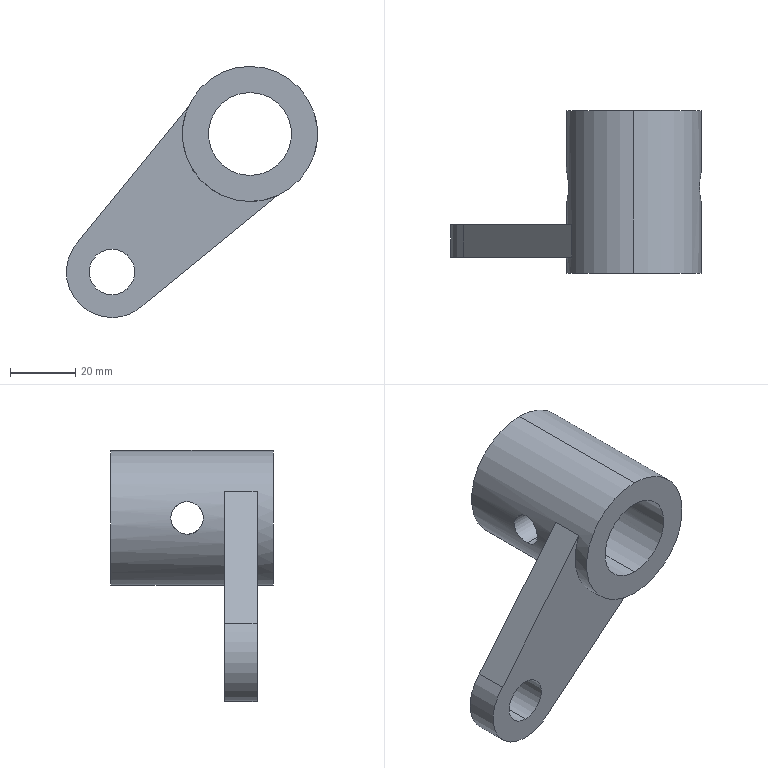Part | SolidWorks | features BaseBody 1 | 1 solid | 18 faces | box 77.176 x 50 x 77.176 mm | volume 56101 mm3 | cylinder 12 | plane 6 | commonest cylinder face diameters 10 x4 14 x2 25.5 x2 28 x2 41.5 x2
STEP:
#1=CARTESIAN_POINT('',(942.084,-3520.973,889.971));
#2=VERTEX_POINT('',#1);
#3=CARTESIAN_POINT('',(942.084,-3520.973,899.971));
#4=VERTEX_POINT('',#3);
#5=CARTESIAN_POINT('',(942.084,-3520.973,889.971));
#6=CARTESIAN_POINT('',(942.084,-3521.305,889.971));
#7=CARTESIAN_POINT('',(942.092,-3521.631,890.004));
#8=CARTESIAN_POINT('',(942.123,-3522.271,890.132));
#9=CARTESIAN_POINT('',(942.147,-3522.589,890.229));
#10=CARTESIAN_POINT('',(942.204,-3523.194,890.48));
#11=CARTESIAN_POINT('',(942.238,-3523.481,890.633));
#12=CARTESIAN_POINT('',(942.312,-3524.023,890.996));
#13=CARTESIAN_POINT('',(942.352,-3524.279,891.206));
#14=CARTESIAN_POINT('',(942.432,-3524.739,891.666));
#15=CARTESIAN_POINT('',(942.471,-3524.945,891.917));
#16=CARTESIAN_POINT('',(942.545,-3525.311,892.463));
#17=CARTESIAN_POINT('',(942.579,-3525.465,892.752));
#18=CARTESIAN_POINT('',(942.635,-3525.715,893.353));
#19=CARTESIAN_POINT('',(942.657,-3525.812,893.669));
#20=CARTESIAN_POINT('',(942.688,-3525.941,894.316));
#21=CARTESIAN_POINT('',(942.696,-3525.973,894.644));
#22=CARTESIAN_POINT('',(942.695,-3525.973,895.307));
#23=CARTESIAN_POINT('',(942.687,-3525.94,895.633));
#24=CARTESIAN_POINT('',(942.657,-3525.812,896.273));
#25=CARTESIAN_POINT('',(942.634,-3525.715,896.591));
#26=CARTESIAN_POINT('',(942.578,-3525.463,897.196));
#27=CARTESIAN_POINT('',(942.545,-3525.309,897.483));
#28=CARTESIAN_POINT('',(942.471,-3524.946,898.025));
#29=CARTESIAN_POINT('',(942.431,-3524.735,898.281));
#30=CARTESIAN_POINT('',(942.352,-3524.276,898.739));
#31=CARTESIAN_POINT('',(942.312,-3524.025,898.946));
#32=CARTESIAN_POINT('',(942.238,-3523.478,899.311));
#33=CARTESIAN_POINT('',(942.203,-3523.189,899.465));
#34=CARTESIAN_POINT('',(942.161,-3522.738,899.652));
#35=CARTESIAN_POINT('',(942.148,-3522.585,899.707));
#36=CARTESIAN_POINT('',(942.125,-3522.271,899.803));
#37=CARTESIAN_POINT('',(942.116,-3522.11,899.843));
#38=CARTESIAN_POINT('',(942.092,-3521.626,899.94));
#39=CARTESIAN_POINT('',(942.084,-3521.301,899.971));
#40=CARTESIAN_POINT('',(942.084,-3520.973,899.971));
#41=B_SPLINE_CURVE_WITH_KNOTS('',3,(#5,#6,#7,#8,#9,#10,#11,#12,#13,#14,#15,#16,#17,#18,#19,#20,#21,#22,#23,#24,#25,#26,#27,#28,#29,#30,#31,#32,#33,#34,#35,#36,#37,#38,#39,#40),.UNSPECIFIED.,.F.,.F.,(4,2,2,2,2,2,2,2,2,2,2,2,2,2,2,2,2,4),(0.02353,0.02451,0.02549,0.02647,0.02745,0.02843,0.02941,0.03039,0.03137,0.03235,0.03333,0.03431,0.03529,0.03627,0.03725,0.03774,0.03823,0.03921),.UNSPECIFIED.);
#42=EDGE_CURVE('',#2,#4,#41,.T.);
#43=ORIENTED_EDGE('',*,*,#42,.T.);
#44=CARTESIAN_POINT('',(942.084,-3520.973,899.971));
#45=CARTESIAN_POINT('',(942.084,-3520.646,899.971));
#46=CARTESIAN_POINT('',(942.092,-3520.313,899.939));
#47=CARTESIAN_POINT('',(942.124,-3519.672,899.81));
#48=CARTESIAN_POINT('',(942.146,-3519.36,899.715));
#49=CARTESIAN_POINT('',(942.204,-3518.753,899.464));
#50=CARTESIAN_POINT('',(942.238,-3518.463,899.308));
#51=CARTESIAN_POINT('',(942.312,-3517.923,898.947));
#52=CARTESIAN_POINT('',(942.352,-3517.669,898.739));
#53=CARTESIAN_POINT('',(942.432,-3517.206,898.275));
#54=CARTESIAN_POINT('',(942.472,-3517.,898.024));
#55=CARTESIAN_POINT('',(942.545,-3516.638,897.484));
#56=CARTESIAN_POINT('',(942.579,-3516.481,897.192));
#57=CARTESIAN_POINT('',(942.635,-3516.231,896.589));
#58=CARTESIAN_POINT('',(942.657,-3516.135,896.277));
#59=CARTESIAN_POINT('',(942.687,-3516.006,895.634));
#60=CARTESIAN_POINT('',(942.696,-3515.973,895.302));
#61=CARTESIAN_POINT('',(942.696,-3515.973,894.639));
#62=CARTESIAN_POINT('',(942.688,-3516.006,894.314));
#63=CARTESIAN_POINT('',(942.657,-3516.134,893.673));
#64=CARTESIAN_POINT('',(942.635,-3516.23,893.355));
#65=CARTESIAN_POINT('',(942.579,-3516.481,892.751));
#66=CARTESIAN_POINT('',(942.545,-3516.635,892.464));
#67=CARTESIAN_POINT('',(942.472,-3516.997,891.922));
#68=CARTESIAN_POINT('',(942.432,-3517.207,891.666));
#69=CARTESIAN_POINT('',(942.353,-3517.666,891.207));
#70=CARTESIAN_POINT('',(942.313,-3517.917,891.));
#71=CARTESIAN_POINT('',(942.238,-3518.463,890.635));
#72=CARTESIAN_POINT('',(942.204,-3518.751,890.48));
#73=CARTESIAN_POINT('',(942.147,-3519.352,890.23));
#74=CARTESIAN_POINT('',(942.124,-3519.668,890.134));
#75=CARTESIAN_POINT('',(942.092,-3520.314,890.004));
#76=CARTESIAN_POINT('',(942.084,-3520.642,889.971));
#77=CARTESIAN_POINT('',(942.084,-3520.973,889.971));
#78=B_SPLINE_CURVE_WITH_KNOTS('',3,(#44,#45,#46,#47,#48,#49,#50,#51,#52,#53,#54,#55,#56,#57,#58,#59,#60,#61,#62,#63,#64,#65,#66,#67,#68,#69,#70,#71,#72,#73,#74,#75,#76,#77),.UNSPECIFIED.,.F.,.F.,(4,2,2,2,2,2,2,2,2,2,2,2,2,2,2,2,4),(0.007847,0.008827,0.009807,0.01079,0.01177,0.01275,0.01373,0.01471,0.01569,0.01667,0.01765,0.01863,0.01961,0.02059,0.02157,0.02255,0.02353),.UNSPECIFIED.);
#79=EDGE_CURVE('',#4,#2,#78,.T.);
#80=ORIENTED_EDGE('',*,*,#79,.T.);
#81=EDGE_LOOP('',(#43,#80));
#82=FACE_BOUND('',#81,.T.);
#83=CARTESIAN_POINT('',(921.946,-3497.473,874.221));
#84=VERTEX_POINT('',#83);
#85=CARTESIAN_POINT('',(921.946,-3497.473,915.721));
#86=VERTEX_POINT('',#85);
#87=CARTESIAN_POINT('',(921.946,-3497.473,894.971));
#88=DIRECTION('',(0.,-1.,0.));
#89=DIRECTION('',(0.,0.,-1.));
#90=AXIS2_PLACEMENT_3D('',#87,#88,#89);
#91=CIRCLE('',#90,20.75);
#92=EDGE_CURVE('',#84,#86,#91,.T.);
#93=ORIENTED_EDGE('',*,*,#92,.T.);
#94=CARTESIAN_POINT('',(921.946,-3547.473,915.721));
#95=VERTEX_POINT('',#94);
#96=CARTESIAN_POINT('',(921.946,-3547.473,915.721));
#97=DIRECTION('',(0.,-1.,0.));
#98=VECTOR('',#97,1000.);
#99=LINE('',#96,#98);
#100=EDGE_CURVE('',#86,#95,#99,.T.);
#101=ORIENTED_EDGE('',*,*,#100,.T.);
#102=CARTESIAN_POINT('',(921.946,-3547.473,874.221));
#103=VERTEX_POINT('',#102);
#104=CARTESIAN_POINT('',(921.946,-3547.473,894.971));
#105=DIRECTION('',(0.,1.,0.));
#106=DIRECTION('',(0.,0.,-1.));
#107=AXIS2_PLACEMENT_3D('',#104,#105,#106);
#108=CIRCLE('',#107,20.75);
#109=EDGE_CURVE('',#95,#103,#108,.T.);
#110=ORIENTED_EDGE('',*,*,#109,.T.);
#111=CARTESIAN_POINT('',(921.946,-3542.473,874.221));
#112=VERTEX_POINT('',#111);
#113=CARTESIAN_POINT('',(921.946,-3547.473,874.221));
#114=DIRECTION('',(0.,-1.,0.));
#115=VECTOR('',#114,1000.);
#116=LINE('',#113,#115);
#117=EDGE_CURVE('',#112,#103,#116,.T.);
#118=ORIENTED_EDGE('',*,*,#117,.F.);
#119=CARTESIAN_POINT('',(930.,-3542.473,875.848));
#120=VERTEX_POINT('',#119);
#121=CARTESIAN_POINT('',(921.946,-3542.473,894.971));
#122=DIRECTION('',(0.,-1.,0.));
#123=DIRECTION('',(0.,0.,-1.));
#124=AXIS2_PLACEMENT_3D('',#121,#122,#123);
#125=CIRCLE('',#124,20.75);
#126=EDGE_CURVE('',#112,#120,#125,.T.);
#127=ORIENTED_EDGE('',*,*,#126,.T.);
#128=CARTESIAN_POINT('',(930.,-3532.473,875.848));
#129=VERTEX_POINT('',#128);
#130=CARTESIAN_POINT('',(930.,-3547.473,875.848));
#131=DIRECTION('',(0.,1.,0.));
#132=VECTOR('',#131,1000.);
#133=LINE('',#130,#132);
#134=EDGE_CURVE('',#120,#129,#133,.T.);
#135=ORIENTED_EDGE('',*,*,#134,.T.);
#136=CARTESIAN_POINT('',(921.946,-3532.473,874.221));
#137=VERTEX_POINT('',#136);
#138=CARTESIAN_POINT('',(921.946,-3532.473,894.971));
#139=DIRECTION('',(0.,1.,0.));
#140=DIRECTION('',(0.,0.,-1.));
#141=AXIS2_PLACEMENT_3D('',#138,#139,#140);
#142=CIRCLE('',#141,20.75);
#143=EDGE_CURVE('',#129,#137,#142,.T.);
#144=ORIENTED_EDGE('',*,*,#143,.T.);
#145=CARTESIAN_POINT('',(921.946,-3547.473,874.221));
#146=DIRECTION('',(0.,-1.,0.));
#147=VECTOR('',#146,1000.);
#148=LINE('',#145,#147);
#149=EDGE_CURVE('',#84,#137,#148,.T.);
#150=ORIENTED_EDGE('',*,*,#149,.F.);
#151=EDGE_LOOP('',(#93,#101,#110,#118,#127,#135,#144,#150));
#152=FACE_OUTER_BOUND('',#151,.T.);
#153=CARTESIAN_POINT('',(921.946,-3547.473,894.971));
#154=DIRECTION('',(0.,-1.,0.));
#155=DIRECTION('',(0.,0.,-1.));
#156=AXIS2_PLACEMENT_3D('',#153,#154,#155);
#157=CYLINDRICAL_SURFACE('',#156,20.75);
#158=ADVANCED_FACE('',(#82,#152),#157,.T.);
#159=CARTESIAN_POINT('',(901.807,-3520.973,899.971));
#160=VERTEX_POINT('',#159);
#161=CARTESIAN_POINT('',(901.807,-3520.973,889.971));
#162=VERTEX_POINT('',#161);
#163=CARTESIAN_POINT('',(901.807,-3520.973,899.971));
#164=CARTESIAN_POINT('',(901.807,-3521.3,899.971));
#165=CARTESIAN_POINT('',(901.799,-3521.633,899.939));
#166=CARTESIAN_POINT('',(901.767,-3522.275,899.81));
#167=CARTESIAN_POINT('',(901.745,-3522.587,899.715));
#168=CARTESIAN_POINT('',(901.687,-3523.193,899.464));
#169=CARTESIAN_POINT('',(901.653,-3523.483,899.308));
#170=CARTESIAN_POINT('',(901.579,-3524.023,898.947));
#171=CARTESIAN_POINT('',(901.539,-3524.277,898.739));
#172=CARTESIAN_POINT('',(901.459,-3524.74,898.275));
#173=CARTESIAN_POINT('',(901.42,-3524.946,898.024));
#174=CARTESIAN_POINT('',(901.346,-3525.308,897.484));
#175=CARTESIAN_POINT('',(901.312,-3525.465,897.192));
#176=CARTESIAN_POINT('',(901.256,-3525.716,896.589));
#177=CARTESIAN_POINT('',(901.234,-3525.811,896.277));
#178=CARTESIAN_POINT('',(901.204,-3525.94,895.634));
#179=CARTESIAN_POINT('',(901.196,-3525.973,895.302));
#180=CARTESIAN_POINT('',(901.196,-3525.973,894.639));
#181=CARTESIAN_POINT('',(901.203,-3525.94,894.314));
#182=CARTESIAN_POINT('',(901.234,-3525.813,893.673));
#183=CARTESIAN_POINT('',(901.256,-3525.716,893.355));
#184=CARTESIAN_POINT('',(901.312,-3525.465,892.751));
#185=CARTESIAN_POINT('',(901.346,-3525.311,892.464));
#186=CARTESIAN_POINT('',(901.419,-3524.949,891.922));
#187=CARTESIAN_POINT('',(901.459,-3524.739,891.666));
#188=CARTESIAN_POINT('',(901.539,-3524.28,891.207));
#189=CARTESIAN_POINT('',(901.578,-3524.029,891.));
#190=CARTESIAN_POINT('',(901.653,-3523.484,890.635));
#191=CARTESIAN_POINT('',(901.687,-3523.195,890.48));
#192=CARTESIAN_POINT('',(901.744,-3522.594,890.23));
#193=CARTESIAN_POINT('',(901.767,-3522.279,890.134));
#194=CARTESIAN_POINT('',(901.799,-3521.632,890.004));
#195=CARTESIAN_POINT('',(901.807,-3521.305,889.971));
#196=CARTESIAN_POINT('',(901.807,-3520.973,889.971));
#197=B_SPLINE_CURVE_WITH_KNOTS('',3,(#163,#164,#165,#166,#167,#168,#169,#170,#171,#172,#173,#174,#175,#176,#177,#178,#179,#180,#181,#182,#183,#184,#185,#186,#187,#188,#189,#190,#191,#192,#193,#194,#195,#196),.UNSPECIFIED.,.F.,.F.,(4,2,2,2,2,2,2,2,2,2,2,2,2,2,2,2,4),(0.007847,0.008827,0.009807,0.01079,0.01177,0.01275,0.01373,0.01471,0.01569,0.01667,0.01765,0.01863,0.01961,0.02059,0.02157,0.02255,0.02353),.UNSPECIFIED.);
#198=EDGE_CURVE('',#160,#162,#197,.T.);
#199=ORIENTED_EDGE('',*,*,#198,.F.);
#200=CARTESIAN_POINT('',(910.217,-3520.973,899.971));
#201=VERTEX_POINT('',#200);
#202=CARTESIAN_POINT('',(883.808,-3520.973,899.971));
#203=DIRECTION('',(1.,0.,0.));
#204=VECTOR('',#203,1000.);
#205=LINE('',#202,#204);
#206=EDGE_CURVE('',#160,#201,#205,.T.);
#207=ORIENTED_EDGE('',*,*,#206,.T.);
#208=CARTESIAN_POINT('',(910.217,-3520.973,889.971));
#209=VERTEX_POINT('',#208);
#210=CARTESIAN_POINT('',(910.217,-3520.973,889.971));
#211=CARTESIAN_POINT('',(910.217,-3521.307,889.971));
#212=CARTESIAN_POINT('',(910.203,-3521.635,890.005));
#213=CARTESIAN_POINT('',(910.149,-3522.278,890.134));
#214=CARTESIAN_POINT('',(910.109,-3522.597,890.231));
#215=CARTESIAN_POINT('',(910.011,-3523.201,890.483));
#216=CARTESIAN_POINT('',(909.953,-3523.487,890.637));
#217=CARTESIAN_POINT('',(909.829,-3524.027,890.999));
#218=CARTESIAN_POINT('',(909.761,-3524.28,891.208));
#219=CARTESIAN_POINT('',(909.63,-3524.737,891.664));
#220=CARTESIAN_POINT('',(909.564,-3524.943,891.914));
#221=CARTESIAN_POINT('',(909.443,-3525.308,892.458));
#222=CARTESIAN_POINT('',(909.388,-3525.462,892.744));
#223=CARTESIAN_POINT('',(909.319,-3525.65,893.195));
#224=CARTESIAN_POINT('',(909.298,-3525.705,893.349));
#225=CARTESIAN_POINT('',(909.262,-3525.802,893.664));
#226=CARTESIAN_POINT('',(909.246,-3525.843,893.825));
#227=CARTESIAN_POINT('',(909.208,-3525.94,894.312));
#228=CARTESIAN_POINT('',(909.195,-3525.973,894.641));
#229=CARTESIAN_POINT('',(909.196,-3525.973,895.309));
#230=CARTESIAN_POINT('',(909.209,-3525.94,895.637));
#231=CARTESIAN_POINT('',(909.259,-3525.81,896.28));
#232=CARTESIAN_POINT('',(909.296,-3525.712,896.6));
#233=CARTESIAN_POINT('',(909.389,-3525.459,897.204));
#234=CARTESIAN_POINT('',(909.444,-3525.305,897.49));
#235=CARTESIAN_POINT('',(909.565,-3524.942,898.031));
#236=CARTESIAN_POINT('',(909.631,-3524.733,898.284));
#237=CARTESIAN_POINT('',(909.763,-3524.276,898.739));
#238=CARTESIAN_POINT('',(909.829,-3524.025,898.945));
#239=CARTESIAN_POINT('',(909.955,-3523.481,899.309));
#240=CARTESIAN_POINT('',(910.012,-3523.195,899.462));
#241=CARTESIAN_POINT('',(910.085,-3522.745,899.65));
#242=CARTESIAN_POINT('',(910.107,-3522.592,899.705));
#243=CARTESIAN_POINT('',(910.146,-3522.277,899.801));
#244=CARTESIAN_POINT('',(910.162,-3522.115,899.842));
#245=CARTESIAN_POINT('',(910.203,-3521.63,899.939));
#246=CARTESIAN_POINT('',(910.217,-3521.303,899.971));
#247=CARTESIAN_POINT('',(910.217,-3520.973,899.971));
#248=B_SPLINE_CURVE_WITH_KNOTS('',3,(#210,#211,#212,#213,#214,#215,#216,#217,#218,#219,#220,#221,#222,#223,#224,#225,#226,#227,#228,#229,#230,#231,#232,#233,#234,#235,#236,#237,#238,#239,#240,#241,#242,#243,#244,#245,#246,#247),.UNSPECIFIED.,.F.,.F.,(4,2,2,2,2,2,2,2,2,2,2,2,2,2,2,2,2,2,4),(-0.007892,-0.006905,-0.005918,-0.004931,-0.003944,-0.002957,-0.00197,-0.001477,-0.0009833,0.000003673,0.0009906,0.001978,0.002964,0.003951,0.004938,0.005925,0.006419,0.006912,0.007899),.UNSPECIFIED.);
#249=EDGE_CURVE('',#209,#201,#248,.T.);
#250=ORIENTED_EDGE('',*,*,#249,.F.);
#251=CARTESIAN_POINT('',(883.808,-3520.973,889.971));
#252=DIRECTION('',(1.,0.,0.));
#253=VECTOR('',#252,1000.);
#254=LINE('',#251,#253);
#255=EDGE_CURVE('',#162,#209,#254,.T.);
#256=ORIENTED_EDGE('',*,*,#255,.F.);
#257=EDGE_LOOP('',(#199,#207,#250,#256));
#258=FACE_OUTER_BOUND('',#257,.T.);
#259=CARTESIAN_POINT('',(883.808,-3520.973,894.971));
#260=DIRECTION('',(1.,0.,0.));
#261=DIRECTION('',(0.,0.,-1.));
#262=AXIS2_PLACEMENT_3D('',#259,#260,#261);
#263=CYLINDRICAL_SURFACE('',#262,5.);
#264=ADVANCED_FACE('',(#258),#263,.F.);
#265=CARTESIAN_POINT('',(933.674,-3520.973,899.971));
#266=VERTEX_POINT('',#265);
#267=CARTESIAN_POINT('',(933.674,-3520.973,889.971));
#268=VERTEX_POINT('',#267);
#269=CARTESIAN_POINT('',(933.674,-3520.973,899.971));
#270=CARTESIAN_POINT('',(933.674,-3521.303,899.971));
#271=CARTESIAN_POINT('',(933.689,-3521.637,899.938));
#272=CARTESIAN_POINT('',(933.743,-3522.281,899.809));
#273=CARTESIAN_POINT('',(933.782,-3522.594,899.713));
#274=CARTESIAN_POINT('',(933.881,-3523.203,899.459));
#275=CARTESIAN_POINT('',(933.938,-3523.489,899.305));
#276=CARTESIAN_POINT('',(934.062,-3524.026,898.944));
#277=CARTESIAN_POINT('',(934.13,-3524.28,898.735));
#278=CARTESIAN_POINT('',(934.262,-3524.738,898.278));
#279=CARTESIAN_POINT('',(934.327,-3524.943,898.029));
#280=CARTESIAN_POINT('',(934.447,-3525.305,897.489));
#281=CARTESIAN_POINT('',(934.503,-3525.462,897.198));
#282=CARTESIAN_POINT('',(934.595,-3525.712,896.598));
#283=CARTESIAN_POINT('',(934.632,-3525.809,896.286));
#284=CARTESIAN_POINT('',(934.682,-3525.94,895.635));
#285=CARTESIAN_POINT('',(934.696,-3525.973,895.304));
#286=CARTESIAN_POINT('',(934.695,-3525.973,894.636));
#287=CARTESIAN_POINT('',(934.682,-3525.94,894.309));
#288=CARTESIAN_POINT('',(934.633,-3525.811,893.665));
#289=CARTESIAN_POINT('',(934.595,-3525.713,893.346));
#290=CARTESIAN_POINT('',(934.503,-3525.461,892.742));
#291=CARTESIAN_POINT('',(934.448,-3525.307,892.457));
#292=CARTESIAN_POINT('',(934.327,-3524.944,891.916));
#293=CARTESIAN_POINT('',(934.261,-3524.736,891.663));
#294=CARTESIAN_POINT('',(934.129,-3524.28,891.207));
#295=CARTESIAN_POINT('',(934.063,-3524.029,891.001));
#296=CARTESIAN_POINT('',(933.938,-3523.486,890.637));
#297=CARTESIAN_POINT('',(933.88,-3523.201,890.483));
#298=CARTESIAN_POINT('',(933.807,-3522.751,890.295));
#299=CARTESIAN_POINT('',(933.785,-3522.598,890.24));
#300=CARTESIAN_POINT('',(933.746,-3522.283,890.143));
#301=CARTESIAN_POINT('',(933.729,-3522.122,890.102));
#302=CARTESIAN_POINT('',(933.689,-3521.636,890.005));
#303=CARTESIAN_POINT('',(933.674,-3521.307,889.971));
#304=CARTESIAN_POINT('',(933.674,-3520.973,889.971));
#305=B_SPLINE_CURVE_WITH_KNOTS('',3,(#269,#270,#271,#272,#273,#274,#275,#276,#277,#278,#279,#280,#281,#282,#283,#284,#285,#286,#287,#288,#289,#290,#291,#292,#293,#294,#295,#296,#297,#298,#299,#300,#301,#302,#303,#304),.UNSPECIFIED.,.F.,.F.,(4,2,2,2,2,2,2,2,2,2,2,2,2,2,2,2,2,4),(0.007899,0.008885,0.009871,0.01086,0.01184,0.01283,0.01382,0.0148,0.01579,0.01677,0.01776,0.01875,0.01973,0.02072,0.0217,0.0222,0.02269,0.02367),.UNSPECIFIED.);
#306=EDGE_CURVE('',#266,#268,#305,.T.);
#307=ORIENTED_EDGE('',*,*,#306,.F.);
#308=CARTESIAN_POINT('',(883.808,-3520.973,899.971));
#309=DIRECTION('',(1.,0.,0.));
#310=VECTOR('',#309,1000.);
#311=LINE('',#308,#310);
#312=EDGE_CURVE('',#266,#4,#311,.T.);
#313=ORIENTED_EDGE('',*,*,#312,.T.);
#314=ORIENTED_EDGE('',*,*,#42,.F.);
#315=CARTESIAN_POINT('',(883.808,-3520.973,889.971));
#316=DIRECTION('',(1.,0.,0.));
#317=VECTOR('',#316,1000.);
#318=LINE('',#315,#317);
#319=EDGE_CURVE('',#268,#2,#318,.T.);
#320=ORIENTED_EDGE('',*,*,#319,.F.);
#321=EDGE_LOOP('',(#307,#313,#314,#320));
#322=FACE_OUTER_BOUND('',#321,.T.);
#323=CARTESIAN_POINT('',(883.808,-3520.973,894.971));
#324=DIRECTION('',(1.,0.,0.));
#325=DIRECTION('',(0.,0.,-1.));
#326=AXIS2_PLACEMENT_3D('',#323,#324,#325);
#327=CYLINDRICAL_SURFACE('',#326,5.);
#328=ADVANCED_FACE('',(#322),#327,.F.);
#329=ORIENTED_EDGE('',*,*,#249,.T.);
#330=CARTESIAN_POINT('',(910.217,-3520.973,899.971));
#331=CARTESIAN_POINT('',(910.217,-3520.644,899.971));
#332=CARTESIAN_POINT('',(910.202,-3520.309,899.938));
#333=CARTESIAN_POINT('',(910.148,-3519.665,899.809));
#334=CARTESIAN_POINT('',(910.109,-3519.352,899.713));
#335=CARTESIAN_POINT('',(910.011,-3518.743,899.459));
#336=CARTESIAN_POINT('',(909.953,-3518.458,899.305));
#337=CARTESIAN_POINT('',(909.829,-3517.92,898.944));
#338=CARTESIAN_POINT('',(909.761,-3517.666,898.735));
#339=CARTESIAN_POINT('',(909.629,-3517.208,898.278));
#340=CARTESIAN_POINT('',(909.564,-3517.004,898.029));
#341=CARTESIAN_POINT('',(909.444,-3516.641,897.489));
#342=CARTESIAN_POINT('',(909.388,-3516.485,897.198));
#343=CARTESIAN_POINT('',(909.296,-3516.234,896.598));
#344=CARTESIAN_POINT('',(909.259,-3516.138,896.286));
#345=CARTESIAN_POINT('',(909.209,-3516.006,895.635));
#346=CARTESIAN_POINT('',(909.195,-3515.973,895.304));
#347=CARTESIAN_POINT('',(909.196,-3515.973,894.636));
#348=CARTESIAN_POINT('',(909.209,-3516.006,894.309));
#349=CARTESIAN_POINT('',(909.258,-3516.136,893.665));
#350=CARTESIAN_POINT('',(909.296,-3516.233,893.346));
#351=CARTESIAN_POINT('',(909.388,-3516.486,892.742));
#352=CARTESIAN_POINT('',(909.443,-3516.639,892.457));
#353=CARTESIAN_POINT('',(909.564,-3517.002,891.916));
#354=CARTESIAN_POINT('',(909.63,-3517.211,891.663));
#355=CARTESIAN_POINT('',(909.762,-3517.667,891.207));
#356=CARTESIAN_POINT('',(909.828,-3517.917,891.001));
#357=CARTESIAN_POINT('',(909.954,-3518.46,890.637));
#358=CARTESIAN_POINT('',(910.011,-3518.745,890.483));
#359=CARTESIAN_POINT('',(910.084,-3519.195,890.295));
#360=CARTESIAN_POINT('',(910.106,-3519.349,890.24));
#361=CARTESIAN_POINT('',(910.145,-3519.663,890.143));
#362=CARTESIAN_POINT('',(910.162,-3519.824,890.102));
#363=CARTESIAN_POINT('',(910.203,-3520.311,890.005));
#364=CARTESIAN_POINT('',(910.217,-3520.639,889.971));
#365=CARTESIAN_POINT('',(910.217,-3520.973,889.971));
#366=B_SPLINE_CURVE_WITH_KNOTS('',3,(#330,#331,#332,#333,#334,#335,#336,#337,#338,#339,#340,#341,#342,#343,#344,#345,#346,#347,#348,#349,#350,#351,#352,#353,#354,#355,#356,#357,#358,#359,#360,#361,#362,#363,#364,#365),.UNSPECIFIED.,.F.,.F.,(4,2,2,2,2,2,2,2,2,2,2,2,2,2,2,2,2,4),(0.007899,0.008885,0.009871,0.01086,0.01184,0.01283,0.01382,0.0148,0.01579,0.01677,0.01776,0.01875,0.01973,0.02072,0.0217,0.0222,0.02269,0.02367),.UNSPECIFIED.);
#367=EDGE_CURVE('',#201,#209,#366,.T.);
#368=ORIENTED_EDGE('',*,*,#367,.T.);
#369=EDGE_LOOP('',(#329,#368));
#370=FACE_BOUND('',#369,.T.);
#371=CARTESIAN_POINT('',(921.946,-3497.473,907.721));
#372=VERTEX_POINT('',#371);
#373=CARTESIAN_POINT('',(921.946,-3497.473,882.221));
#374=VERTEX_POINT('',#373);
#375=CARTESIAN_POINT('',(921.946,-3497.473,894.971));
#376=DIRECTION('',(0.,-1.,0.));
#377=DIRECTION('',(0.,0.,-1.));
#378=AXIS2_PLACEMENT_3D('',#375,#376,#377);
#379=CIRCLE('',#378,12.75);
#380=EDGE_CURVE('',#372,#374,#379,.T.);
#381=ORIENTED_EDGE('',*,*,#380,.F.);
#382=CARTESIAN_POINT('',(921.946,-3547.473,907.721));
#383=VERTEX_POINT('',#382);
#384=CARTESIAN_POINT('',(921.946,-3497.473,907.721));
#385=DIRECTION('',(0.,-1.,0.));
#386=VECTOR('',#385,1000.);
#387=LINE('',#384,#386);
#388=EDGE_CURVE('',#372,#383,#387,.T.);
#389=ORIENTED_EDGE('',*,*,#388,.T.);
#390=CARTESIAN_POINT('',(921.946,-3547.473,882.221));
#391=VERTEX_POINT('',#390);
#392=CARTESIAN_POINT('',(921.946,-3547.473,894.971));
#393=DIRECTION('',(0.,-1.,0.));
#394=DIRECTION('',(0.,0.,-1.));
#395=AXIS2_PLACEMENT_3D('',#392,#393,#394);
#396=CIRCLE('',#395,12.75);
#397=EDGE_CURVE('',#383,#391,#396,.T.);
#398=ORIENTED_EDGE('',*,*,#397,.T.);
#399=CARTESIAN_POINT('',(921.946,-3497.473,882.221));
#400=DIRECTION('',(0.,-1.,0.));
#401=VECTOR('',#400,1000.);
#402=LINE('',#399,#401);
#403=EDGE_CURVE('',#374,#391,#402,.T.);
#404=ORIENTED_EDGE('',*,*,#403,.F.);
#405=EDGE_LOOP('',(#381,#389,#398,#404));
#406=FACE_OUTER_BOUND('',#405,.T.);
#407=CARTESIAN_POINT('',(921.946,-3497.473,894.971));
#408=DIRECTION('',(0.,-1.,0.));
#409=DIRECTION('',(0.,0.,-1.));
#410=AXIS2_PLACEMENT_3D('',#407,#408,#409);
#411=CYLINDRICAL_SURFACE('',#410,12.75);
#412=ADVANCED_FACE('',(#370,#406),#411,.F.);
#413=CARTESIAN_POINT('',(879.519,-3532.473,845.545));
#414=VERTEX_POINT('',#413);
#415=CARTESIAN_POINT('',(879.519,-3532.473,859.545));
#416=VERTEX_POINT('',#415);
#417=CARTESIAN_POINT('',(879.519,-3532.473,852.545));
#418=DIRECTION('',(0.,1.,0.));
#419=DIRECTION('',(0.,0.,-1.));
#420=AXIS2_PLACEMENT_3D('',#417,#418,#419);
#421=CIRCLE('',#420,7.);
#422=EDGE_CURVE('',#414,#416,#421,.T.);
#423=ORIENTED_EDGE('',*,*,#422,.T.);
#424=CARTESIAN_POINT('',(879.519,-3542.473,859.545));
#425=VERTEX_POINT('',#424);
#426=CARTESIAN_POINT('',(879.519,-3532.473,859.545));
#427=DIRECTION('',(0.,-1.,0.));
#428=VECTOR('',#427,1000.);
#429=LINE('',#426,#428);
#430=EDGE_CURVE('',#416,#425,#429,.T.);
#431=ORIENTED_EDGE('',*,*,#430,.T.);
#432=CARTESIAN_POINT('',(879.519,-3542.473,845.545));
#433=VERTEX_POINT('',#432);
#434=CARTESIAN_POINT('',(879.519,-3542.473,852.545));
#435=DIRECTION('',(0.,1.,0.));
#436=DIRECTION('',(0.,0.,-1.));
#437=AXIS2_PLACEMENT_3D('',#434,#435,#436);
#438=CIRCLE('',#437,7.);
#439=EDGE_CURVE('',#433,#425,#438,.T.);
#440=ORIENTED_EDGE('',*,*,#439,.F.);
#441=CARTESIAN_POINT('',(879.519,-3532.473,845.545));
#442=DIRECTION('',(0.,-1.,0.));
#443=VECTOR('',#442,1000.);
#444=LINE('',#441,#443);
#445=EDGE_CURVE('',#414,#433,#444,.T.);
#446=ORIENTED_EDGE('',*,*,#445,.F.);
#447=EDGE_LOOP('',(#423,#431,#440,#446));
#448=FACE_OUTER_BOUND('',#447,.T.);
#449=CARTESIAN_POINT('',(879.519,-3532.473,852.545));
#450=DIRECTION('',(0.,-1.,0.));
#451=DIRECTION('',(0.,0.,-1.));
#452=AXIS2_PLACEMENT_3D('',#449,#450,#451);
#453=CYLINDRICAL_SURFACE('',#452,7.);
#454=ADVANCED_FACE('',(#448),#453,.F.);
#455=CARTESIAN_POINT('',(869.62,-3532.473,862.445));
#456=VERTEX_POINT('',#455);
#457=CARTESIAN_POINT('',(879.519,-3532.473,838.545));
#458=VERTEX_POINT('',#457);
#459=CARTESIAN_POINT('',(879.519,-3532.473,852.545));
#460=DIRECTION('',(0.,-1.,0.));
#461=DIRECTION('',(0.,0.,-1.));
#462=AXIS2_PLACEMENT_3D('',#459,#460,#461);
#463=CIRCLE('',#462,14.);
#464=EDGE_CURVE('',#456,#458,#463,.T.);
#465=ORIENTED_EDGE('',*,*,#464,.T.);
#466=CARTESIAN_POINT('',(879.519,-3542.473,838.545));
#467=VERTEX_POINT('',#466);
#468=CARTESIAN_POINT('',(879.519,-3542.473,838.545));
#469=DIRECTION('',(0.,-1.,0.));
#470=VECTOR('',#469,1000.);
#471=LINE('',#468,#470);
#472=EDGE_CURVE('',#458,#467,#471,.T.);
#473=ORIENTED_EDGE('',*,*,#472,.T.);
#474=CARTESIAN_POINT('',(869.62,-3542.473,862.445));
#475=VERTEX_POINT('',#474);
#476=CARTESIAN_POINT('',(879.519,-3542.473,852.545));
#477=DIRECTION('',(0.,-1.,0.));
#478=DIRECTION('',(0.,0.,-1.));
#479=AXIS2_PLACEMENT_3D('',#476,#477,#478);
#480=CIRCLE('',#479,14.);
#481=EDGE_CURVE('',#475,#467,#480,.T.);
#482=ORIENTED_EDGE('',*,*,#481,.F.);
#483=CARTESIAN_POINT('',(869.62,-3542.473,862.445));
#484=DIRECTION('',(0.,-1.,0.));
#485=VECTOR('',#484,1000.);
#486=LINE('',#483,#485);
#487=EDGE_CURVE('',#456,#475,#486,.T.);
#488=ORIENTED_EDGE('',*,*,#487,.F.);
#489=EDGE_LOOP('',(#465,#473,#482,#488));
#490=FACE_OUTER_BOUND('',#489,.T.);
#491=CARTESIAN_POINT('',(879.519,-3542.473,852.545));
#492=DIRECTION('',(0.,-1.,0.));
#493=DIRECTION('',(0.,0.,-1.));
#494=AXIS2_PLACEMENT_3D('',#491,#492,#493);
#495=CYLINDRICAL_SURFACE('',#494,14.);
#496=ADVANCED_FACE('',(#490),#495,.T.);
#497=ORIENTED_EDGE('',*,*,#100,.F.);
#498=CARTESIAN_POINT('',(921.946,-3497.473,894.971));
#499=DIRECTION('',(0.,-1.,0.));
#500=DIRECTION('',(0.,0.,-1.));
#501=AXIS2_PLACEMENT_3D('',#498,#499,#500);
#502=CIRCLE('',#501,20.75);
#503=EDGE_CURVE('',#86,#84,#502,.T.);
#504=ORIENTED_EDGE('',*,*,#503,.T.);
#505=ORIENTED_EDGE('',*,*,#149,.T.);
#506=CARTESIAN_POINT('',(902.823,-3532.473,903.026));
#507=VERTEX_POINT('',#506);
#508=CARTESIAN_POINT('',(921.946,-3532.473,894.971));
#509=DIRECTION('',(0.,1.,0.));
#510=DIRECTION('',(0.,0.,-1.));
#511=AXIS2_PLACEMENT_3D('',#508,#509,#510);
#512=CIRCLE('',#511,20.75);
#513=EDGE_CURVE('',#137,#507,#512,.T.);
#514=ORIENTED_EDGE('',*,*,#513,.T.);
#515=CARTESIAN_POINT('',(902.823,-3542.473,903.026));
#516=VERTEX_POINT('',#515);
#517=CARTESIAN_POINT('',(902.823,-3547.473,903.026));
#518=DIRECTION('',(0.,-1.,0.));
#519=VECTOR('',#518,1000.);
#520=LINE('',#517,#519);
#521=EDGE_CURVE('',#507,#516,#520,.T.);
#522=ORIENTED_EDGE('',*,*,#521,.T.);
#523=CARTESIAN_POINT('',(921.946,-3542.473,894.971));
#524=DIRECTION('',(0.,-1.,0.));
#525=DIRECTION('',(0.,0.,-1.));
#526=AXIS2_PLACEMENT_3D('',#523,#524,#525);
#527=CIRCLE('',#526,20.75);
#528=EDGE_CURVE('',#516,#112,#527,.T.);
#529=ORIENTED_EDGE('',*,*,#528,.T.);
#530=ORIENTED_EDGE('',*,*,#117,.T.);
#531=CARTESIAN_POINT('',(921.946,-3547.473,894.971));
#532=DIRECTION('',(0.,1.,0.));
#533=DIRECTION('',(0.,0.,-1.));
#534=AXIS2_PLACEMENT_3D('',#531,#532,#533);
#535=CIRCLE('',#534,20.75);
#536=EDGE_CURVE('',#103,#95,#535,.T.);
#537=ORIENTED_EDGE('',*,*,#536,.T.);
#538=EDGE_LOOP('',(#497,#504,#505,#514,#522,#529,#530,#537));
#539=FACE_OUTER_BOUND('',#538,.T.);
#540=CARTESIAN_POINT('',(901.807,-3520.973,889.971));
#541=CARTESIAN_POINT('',(901.807,-3520.642,889.971));
#542=CARTESIAN_POINT('',(901.799,-3520.316,890.004));
#543=CARTESIAN_POINT('',(901.768,-3519.675,890.132));
#544=CARTESIAN_POINT('',(901.744,-3519.357,890.229));
#545=CARTESIAN_POINT('',(901.687,-3518.752,890.48));
#546=CARTESIAN_POINT('',(901.653,-3518.465,890.633));
#547=CARTESIAN_POINT('',(901.579,-3517.923,890.996));
#548=CARTESIAN_POINT('',(901.539,-3517.667,891.206));
#549=CARTESIAN_POINT('',(901.459,-3517.208,891.666));
#550=CARTESIAN_POINT('',(901.42,-3517.001,891.917));
#551=CARTESIAN_POINT('',(901.346,-3516.636,892.463));
#552=CARTESIAN_POINT('',(901.312,-3516.481,892.752));
#553=CARTESIAN_POINT('',(901.257,-3516.231,893.353));
#554=CARTESIAN_POINT('',(901.234,-3516.135,893.669));
#555=CARTESIAN_POINT('',(901.203,-3516.005,894.316));
#556=CARTESIAN_POINT('',(901.195,-3515.973,894.644));
#557=CARTESIAN_POINT('',(901.196,-3515.973,895.307));
#558=CARTESIAN_POINT('',(901.204,-3516.006,895.633));
#559=CARTESIAN_POINT('',(901.234,-3516.134,896.273));
#560=CARTESIAN_POINT('',(901.257,-3516.231,896.591));
#561=CARTESIAN_POINT('',(901.313,-3516.483,897.196));
#562=CARTESIAN_POINT('',(901.346,-3516.637,897.483));
#563=CARTESIAN_POINT('',(901.42,-3517.,898.025));
#564=CARTESIAN_POINT('',(901.46,-3517.211,898.281));
#565=CARTESIAN_POINT('',(901.539,-3517.67,898.739));
#566=CARTESIAN_POINT('',(901.579,-3517.922,898.946));
#567=CARTESIAN_POINT('',(901.654,-3518.468,899.311));
#568=CARTESIAN_POINT('',(901.688,-3518.757,899.465));
#569=CARTESIAN_POINT('',(901.73,-3519.208,899.652));
#570=CARTESIAN_POINT('',(901.743,-3519.361,899.707));
#571=CARTESIAN_POINT('',(901.766,-3519.675,899.803));
#572=CARTESIAN_POINT('',(901.776,-3519.836,899.843));
#573=CARTESIAN_POINT('',(901.799,-3520.321,899.94));
#574=CARTESIAN_POINT('',(901.807,-3520.646,899.971));
#575=CARTESIAN_POINT('',(901.807,-3520.973,899.971));
#576=B_SPLINE_CURVE_WITH_KNOTS('',3,(#540,#541,#542,#543,#544,#545,#546,#547,#548,#549,#550,#551,#552,#553,#554,#555,#556,#557,#558,#559,#560,#561,#562,#563,#564,#565,#566,#567,#568,#569,#570,#571,#572,#573,#574,#575),.UNSPECIFIED.,.F.,.F.,(4,2,2,2,2,2,2,2,2,2,2,2,2,2,2,2,2,4),(0.02353,0.02451,0.02549,0.02647,0.02745,0.02843,0.02941,0.03039,0.03137,0.03235,0.03333,0.03431,0.03529,0.03627,0.03725,0.03774,0.03823,0.03921),.UNSPECIFIED.);
#577=EDGE_CURVE('',#162,#160,#576,.T.);
#578=ORIENTED_EDGE('',*,*,#577,.T.);
#579=ORIENTED_EDGE('',*,*,#198,.T.);
#580=EDGE_LOOP('',(#578,#579));
#581=FACE_BOUND('',#580,.T.);
#582=CARTESIAN_POINT('',(921.946,-3547.473,894.971));
#583=DIRECTION('',(0.,-1.,0.));
#584=DIRECTION('',(0.,0.,-1.));
#585=AXIS2_PLACEMENT_3D('',#582,#583,#584);
#586=CYLINDRICAL_SURFACE('',#585,20.75);
#587=ADVANCED_FACE('',(#539,#581),#586,.T.);
#588=ORIENTED_EDGE('',*,*,#536,.F.);
#589=ORIENTED_EDGE('',*,*,#109,.F.);
#590=EDGE_LOOP('',(#588,#589));
#591=FACE_OUTER_BOUND('',#590,.T.);
#592=CARTESIAN_POINT('',(921.946,-3547.473,894.971));
#593=DIRECTION('',(0.,-1.,0.));
#594=DIRECTION('',(0.,0.,-1.));
#595=AXIS2_PLACEMENT_3D('',#592,#593,#594);
#596=CIRCLE('',#595,12.75);
#597=EDGE_CURVE('',#391,#383,#596,.T.);
#598=ORIENTED_EDGE('',*,*,#597,.F.);
#599=ORIENTED_EDGE('',*,*,#397,.F.);
#600=EDGE_LOOP('',(#598,#599));
#601=FACE_BOUND('',#600,.T.);
#602=CARTESIAN_POINT('',(921.946,-3547.473,894.971));
#603=DIRECTION('',(0.,1.,0.));
#604=DIRECTION('',(0.,0.,1.));
#605=AXIS2_PLACEMENT_3D('',#602,#603,#604);
#606=PLANE('',#605);
#607=ADVANCED_FACE('',(#591,#601),#606,.F.);
#608=ORIENTED_EDGE('',*,*,#439,.T.);
#609=CARTESIAN_POINT('',(879.519,-3542.473,852.545));
#610=DIRECTION('',(0.,1.,0.));
#611=DIRECTION('',(0.,0.,-1.));
#612=AXIS2_PLACEMENT_3D('',#609,#610,#611);
#613=CIRCLE('',#612,7.);
#614=EDGE_CURVE('',#425,#433,#613,.T.);
#615=ORIENTED_EDGE('',*,*,#614,.T.);
#616=EDGE_LOOP('',(#608,#615));
#617=FACE_BOUND('',#616,.T.);
#618=CARTESIAN_POINT('',(889.419,-3542.473,842.646));
#619=VERTEX_POINT('',#618);
#620=CARTESIAN_POINT('',(889.419,-3542.473,842.646));
#621=DIRECTION('',(0.774,0.,0.6332));
#622=VECTOR('',#621,1000.);
#623=LINE('',#620,#622);
#624=EDGE_CURVE('',#619,#120,#623,.T.);
#625=ORIENTED_EDGE('',*,*,#624,.T.);
#626=ORIENTED_EDGE('',*,*,#126,.F.);
#627=ORIENTED_EDGE('',*,*,#528,.F.);
#628=CARTESIAN_POINT('',(902.823,-3542.473,903.026));
#629=DIRECTION('',(-0.6332,0.,-0.774));
#630=VECTOR('',#629,1000.);
#631=LINE('',#628,#630);
#632=EDGE_CURVE('',#516,#475,#631,.T.);
#633=ORIENTED_EDGE('',*,*,#632,.T.);
#634=ORIENTED_EDGE('',*,*,#481,.T.);
#635=CARTESIAN_POINT('',(879.519,-3542.473,852.545));
#636=DIRECTION('',(0.,-1.,0.));
#637=DIRECTION('',(0.,0.,-1.));
#638=AXIS2_PLACEMENT_3D('',#635,#636,#637);
#639=CIRCLE('',#638,14.);
#640=EDGE_CURVE('',#467,#619,#639,.T.);
#641=ORIENTED_EDGE('',*,*,#640,.T.);
#642=EDGE_LOOP('',(#625,#626,#627,#633,#634,#641));
#643=FACE_OUTER_BOUND('',#642,.T.);
#644=CARTESIAN_POINT('',(903.556,-3542.473,876.582));
#645=DIRECTION('',(0.,-1.,0.));
#646=DIRECTION('',(1.,0.,0.));
#647=AXIS2_PLACEMENT_3D('',#644,#645,#646);
#648=PLANE('',#647);
#649=ADVANCED_FACE('',(#617,#643),#648,.T.);
#650=ORIENTED_EDGE('',*,*,#487,.T.);
#651=ORIENTED_EDGE('',*,*,#632,.F.);
#652=ORIENTED_EDGE('',*,*,#521,.F.);
#653=CARTESIAN_POINT('',(869.62,-3532.473,862.445));
#654=DIRECTION('',(-0.6332,0.,-0.774));
#655=VECTOR('',#654,1000.);
#656=LINE('',#653,#655);
#657=EDGE_CURVE('',#507,#456,#656,.T.);
#658=ORIENTED_EDGE('',*,*,#657,.T.);
#659=EDGE_LOOP('',(#650,#651,#652,#658));
#660=FACE_OUTER_BOUND('',#659,.T.);
#661=CARTESIAN_POINT('',(869.62,-3542.473,862.445));
#662=DIRECTION('',(-0.774,0.,0.6332));
#663=DIRECTION('',(0.6332,0.,0.774));
#664=AXIS2_PLACEMENT_3D('',#661,#662,#663);
#665=PLANE('',#664);
#666=ADVANCED_FACE('',(#660),#665,.T.);
#667=ORIENTED_EDGE('',*,*,#422,.F.);
#668=CARTESIAN_POINT('',(879.519,-3532.473,852.545));
#669=DIRECTION('',(0.,1.,0.));
#670=DIRECTION('',(0.,0.,-1.));
#671=AXIS2_PLACEMENT_3D('',#668,#669,#670);
#672=CIRCLE('',#671,7.);
#673=EDGE_CURVE('',#416,#414,#672,.T.);
#674=ORIENTED_EDGE('',*,*,#673,.F.);
#675=EDGE_LOOP('',(#667,#674));
#676=FACE_BOUND('',#675,.T.);
#677=CARTESIAN_POINT('',(889.419,-3532.473,842.646));
#678=VERTEX_POINT('',#677);
#679=CARTESIAN_POINT('',(889.419,-3532.473,842.646));
#680=DIRECTION('',(0.774,0.,0.6332));
#681=VECTOR('',#680,1000.);
#682=LINE('',#679,#681);
#683=EDGE_CURVE('',#678,#129,#682,.T.);
#684=ORIENTED_EDGE('',*,*,#683,.F.);
#685=CARTESIAN_POINT('',(879.519,-3532.473,852.545));
#686=DIRECTION('',(0.,-1.,0.));
#687=DIRECTION('',(0.,0.,-1.));
#688=AXIS2_PLACEMENT_3D('',#685,#686,#687);
#689=CIRCLE('',#688,14.);
#690=EDGE_CURVE('',#458,#678,#689,.T.);
#691=ORIENTED_EDGE('',*,*,#690,.F.);
#692=ORIENTED_EDGE('',*,*,#464,.F.);
#693=ORIENTED_EDGE('',*,*,#657,.F.);
#694=ORIENTED_EDGE('',*,*,#513,.F.);
#695=ORIENTED_EDGE('',*,*,#143,.F.);
#696=EDGE_LOOP('',(#684,#691,#692,#693,#694,#695));
#697=FACE_OUTER_BOUND('',#696,.T.);
#698=CARTESIAN_POINT('',(903.556,-3532.473,876.582));
#699=DIRECTION('',(0.,-1.,0.));
#700=DIRECTION('',(1.,0.,0.));
#701=AXIS2_PLACEMENT_3D('',#698,#699,#700);
#702=PLANE('',#701);
#703=ADVANCED_FACE('',(#676,#697),#702,.F.);
#704=ORIENTED_EDGE('',*,*,#206,.F.);
#705=ORIENTED_EDGE('',*,*,#577,.F.);
#706=ORIENTED_EDGE('',*,*,#255,.T.);
#707=ORIENTED_EDGE('',*,*,#367,.F.);
#708=EDGE_LOOP('',(#704,#705,#706,#707));
#709=FACE_OUTER_BOUND('',#708,.T.);
#710=CARTESIAN_POINT('',(883.808,-3520.973,894.971));
#711=DIRECTION('',(1.,0.,0.));
#712=DIRECTION('',(0.,0.,-1.));
#713=AXIS2_PLACEMENT_3D('',#710,#711,#712);
#714=CYLINDRICAL_SURFACE('',#713,5.);
#715=ADVANCED_FACE('',(#709),#714,.F.);
#716=ORIENTED_EDGE('',*,*,#92,.F.);
#717=ORIENTED_EDGE('',*,*,#503,.F.);
#718=EDGE_LOOP('',(#716,#717));
#719=FACE_OUTER_BOUND('',#718,.T.);
#720=CARTESIAN_POINT('',(921.946,-3497.473,894.971));
#721=DIRECTION('',(0.,-1.,0.));
#722=DIRECTION('',(0.,0.,-1.));
#723=AXIS2_PLACEMENT_3D('',#720,#721,#722);
#724=CIRCLE('',#723,12.75);
#725=EDGE_CURVE('',#374,#372,#724,.T.);
#726=ORIENTED_EDGE('',*,*,#725,.T.);
#727=ORIENTED_EDGE('',*,*,#380,.T.);
#728=EDGE_LOOP('',(#726,#727));
#729=FACE_BOUND('',#728,.T.);
#730=CARTESIAN_POINT('',(921.946,-3497.473,894.971));
#731=DIRECTION('',(0.,1.,0.));
#732=DIRECTION('',(0.,0.,1.));
#733=AXIS2_PLACEMENT_3D('',#730,#731,#732);
#734=PLANE('',#733);
#735=ADVANCED_FACE('',(#719,#729),#734,.T.);
#736=ORIENTED_EDGE('',*,*,#312,.F.);
#737=CARTESIAN_POINT('',(933.674,-3520.973,889.971));
#738=CARTESIAN_POINT('',(933.674,-3520.639,889.971));
#739=CARTESIAN_POINT('',(933.689,-3520.312,890.005));
#740=CARTESIAN_POINT('',(933.742,-3519.668,890.134));
#741=CARTESIAN_POINT('',(933.782,-3519.349,890.231));
#742=CARTESIAN_POINT('',(933.88,-3518.745,890.483));
#743=CARTESIAN_POINT('',(933.938,-3518.46,890.637));
#744=CARTESIAN_POINT('',(934.063,-3517.919,890.999));
#745=CARTESIAN_POINT('',(934.13,-3517.666,891.208));
#746=CARTESIAN_POINT('',(934.261,-3517.21,891.664));
#747=CARTESIAN_POINT('',(934.327,-3517.003,891.914));
#748=CARTESIAN_POINT('',(934.449,-3516.638,892.458));
#749=CARTESIAN_POINT('',(934.503,-3516.485,892.744));
#750=CARTESIAN_POINT('',(934.572,-3516.297,893.195));
#751=CARTESIAN_POINT('',(934.593,-3516.241,893.349));
#752=CARTESIAN_POINT('',(934.629,-3516.144,893.664));
#753=CARTESIAN_POINT('',(934.645,-3516.103,893.825));
#754=CARTESIAN_POINT('',(934.683,-3516.006,894.312));
#755=CARTESIAN_POINT('',(934.696,-3515.973,894.641));
#756=CARTESIAN_POINT('',(934.695,-3515.973,895.309));
#757=CARTESIAN_POINT('',(934.682,-3516.007,895.637));
#758=CARTESIAN_POINT('',(934.632,-3516.136,896.28));
#759=CARTESIAN_POINT('',(934.595,-3516.234,896.6));
#760=CARTESIAN_POINT('',(934.502,-3516.487,897.204));
#761=CARTESIAN_POINT('',(934.447,-3516.641,897.49));
#762=CARTESIAN_POINT('',(934.326,-3517.005,898.031));
#763=CARTESIAN_POINT('',(934.26,-3517.214,898.284));
#764=CARTESIAN_POINT('',(934.128,-3517.671,898.739));
#765=CARTESIAN_POINT('',(934.062,-3517.921,898.945));
#766=CARTESIAN_POINT('',(933.937,-3518.465,899.309));
#767=CARTESIAN_POINT('',(933.879,-3518.751,899.462));
#768=CARTESIAN_POINT('',(933.806,-3519.201,899.65));
#769=CARTESIAN_POINT('',(933.784,-3519.355,899.705));
#770=CARTESIAN_POINT('',(933.745,-3519.669,899.801));
#771=CARTESIAN_POINT('',(933.729,-3519.831,899.842));
#772=CARTESIAN_POINT('',(933.688,-3520.316,899.939));
#773=CARTESIAN_POINT('',(933.674,-3520.643,899.971));
#774=CARTESIAN_POINT('',(933.674,-3520.973,899.971));
#775=B_SPLINE_CURVE_WITH_KNOTS('',3,(#737,#738,#739,#740,#741,#742,#743,#744,#745,#746,#747,#748,#749,#750,#751,#752,#753,#754,#755,#756,#757,#758,#759,#760,#761,#762,#763,#764,#765,#766,#767,#768,#769,#770,#771,#772,#773,#774),.UNSPECIFIED.,.F.,.F.,(4,2,2,2,2,2,2,2,2,2,2,2,2,2,2,2,2,2,4),(-0.007892,-0.006905,-0.005918,-0.004931,-0.003944,-0.002957,-0.00197,-0.001477,-0.0009833,0.000003673,0.0009906,0.001978,0.002964,0.003951,0.004938,0.005925,0.006419,0.006912,0.007899),.UNSPECIFIED.);
#776=EDGE_CURVE('',#268,#266,#775,.T.);
#777=ORIENTED_EDGE('',*,*,#776,.F.);
#778=ORIENTED_EDGE('',*,*,#319,.T.);
#779=ORIENTED_EDGE('',*,*,#79,.F.);
#780=EDGE_LOOP('',(#736,#777,#778,#779));
#781=FACE_OUTER_BOUND('',#780,.T.);
#782=CARTESIAN_POINT('',(883.808,-3520.973,894.971));
#783=DIRECTION('',(1.,0.,0.));
#784=DIRECTION('',(0.,0.,-1.));
#785=AXIS2_PLACEMENT_3D('',#782,#783,#784);
#786=CYLINDRICAL_SURFACE('',#785,5.);
#787=ADVANCED_FACE('',(#781),#786,.F.);
#788=ORIENTED_EDGE('',*,*,#388,.F.);
#789=ORIENTED_EDGE('',*,*,#725,.F.);
#790=ORIENTED_EDGE('',*,*,#403,.T.);
#791=ORIENTED_EDGE('',*,*,#597,.T.);
#792=EDGE_LOOP('',(#788,#789,#790,#791));
#793=FACE_OUTER_BOUND('',#792,.T.);
#794=ORIENTED_EDGE('',*,*,#776,.T.);
#795=ORIENTED_EDGE('',*,*,#306,.T.);
#796=EDGE_LOOP('',(#794,#795));
#797=FACE_BOUND('',#796,.T.);
#798=CARTESIAN_POINT('',(921.946,-3497.473,894.971));
#799=DIRECTION('',(0.,-1.,0.));
#800=DIRECTION('',(0.,0.,-1.));
#801=AXIS2_PLACEMENT_3D('',#798,#799,#800);
#802=CYLINDRICAL_SURFACE('',#801,12.75);
#803=ADVANCED_FACE('',(#793,#797),#802,.F.);
#804=CARTESIAN_POINT('',(889.419,-3542.473,842.646));
#805=DIRECTION('',(0.,1.,0.));
#806=VECTOR('',#805,1000.);
#807=LINE('',#804,#806);
#808=EDGE_CURVE('',#619,#678,#807,.T.);
#809=ORIENTED_EDGE('',*,*,#808,.T.);
#810=ORIENTED_EDGE('',*,*,#683,.T.);
#811=ORIENTED_EDGE('',*,*,#134,.F.);
#812=ORIENTED_EDGE('',*,*,#624,.F.);
#813=EDGE_LOOP('',(#809,#810,#811,#812));
#814=FACE_OUTER_BOUND('',#813,.T.);
#815=CARTESIAN_POINT('',(933.007,-3542.473,878.309));
#816=DIRECTION('',(0.6332,0.,-0.774));
#817=DIRECTION('',(-0.774,0.,-0.6332));
#818=AXIS2_PLACEMENT_3D('',#815,#816,#817);
#819=PLANE('',#818);
#820=ADVANCED_FACE('',(#814),#819,.T.);
#821=ORIENTED_EDGE('',*,*,#430,.F.);
#822=ORIENTED_EDGE('',*,*,#673,.T.);
#823=ORIENTED_EDGE('',*,*,#445,.T.);
#824=ORIENTED_EDGE('',*,*,#614,.F.);
#825=EDGE_LOOP('',(#821,#822,#823,#824));
#826=FACE_OUTER_BOUND('',#825,.T.);
#827=CARTESIAN_POINT('',(879.519,-3532.473,852.545));
#828=DIRECTION('',(0.,-1.,0.));
#829=DIRECTION('',(0.,0.,-1.));
#830=AXIS2_PLACEMENT_3D('',#827,#828,#829);
#831=CYLINDRICAL_SURFACE('',#830,7.);
#832=ADVANCED_FACE('',(#826),#831,.F.);
#833=ORIENTED_EDGE('',*,*,#472,.F.);
#834=ORIENTED_EDGE('',*,*,#690,.T.);
#835=ORIENTED_EDGE('',*,*,#808,.F.);
#836=ORIENTED_EDGE('',*,*,#640,.F.);
#837=EDGE_LOOP('',(#833,#834,#835,#836));
#838=FACE_OUTER_BOUND('',#837,.T.);
#839=CARTESIAN_POINT('',(879.519,-3542.473,852.545));
#840=DIRECTION('',(0.,-1.,0.));
#841=DIRECTION('',(0.,0.,-1.));
#842=AXIS2_PLACEMENT_3D('',#839,#840,#841);
#843=CYLINDRICAL_SURFACE('',#842,14.);
#844=ADVANCED_FACE('',(#838),#843,.T.);
#845=CLOSED_SHELL('',(#158,#264,#328,#412,#454,#496,#587,#607,#649,#666,#703,#715,#735,#787,#803,#820,#832,#844));
#846=MANIFOLD_SOLID_BREP('',#845);
#847=CARTESIAN_POINT('',(0.,0.,0.));
#848=DIRECTION('',(0.,0.,1.));
#849=DIRECTION('',(1.,0.,0.));
#850=AXIS2_PLACEMENT_3D('',#847,#848,#849);
#851=(LENGTH_UNIT()NAMED_UNIT(*)SI_UNIT(.MILLI.,.METRE.));
#852=UNCERTAINTY_MEASURE_WITH_UNIT(LENGTH_MEASURE(0.00001),#851,'','');
#853=(NAMED_UNIT(*)PLANE_ANGLE_UNIT()SI_UNIT($,.RADIAN.));
#854=(NAMED_UNIT(*)SI_UNIT($,.STERADIAN.)SOLID_ANGLE_UNIT());
#855=(GEOMETRIC_REPRESENTATION_CONTEXT(3)GLOBAL_UNCERTAINTY_ASSIGNED_CONTEXT((#852))GLOBAL_UNIT_ASSIGNED_CONTEXT((#851,#853,#854))REPRESENTATION_CONTEXT('',''));
#856=ADVANCED_BREP_SHAPE_REPRESENTATION('',(#846,#850),#855);